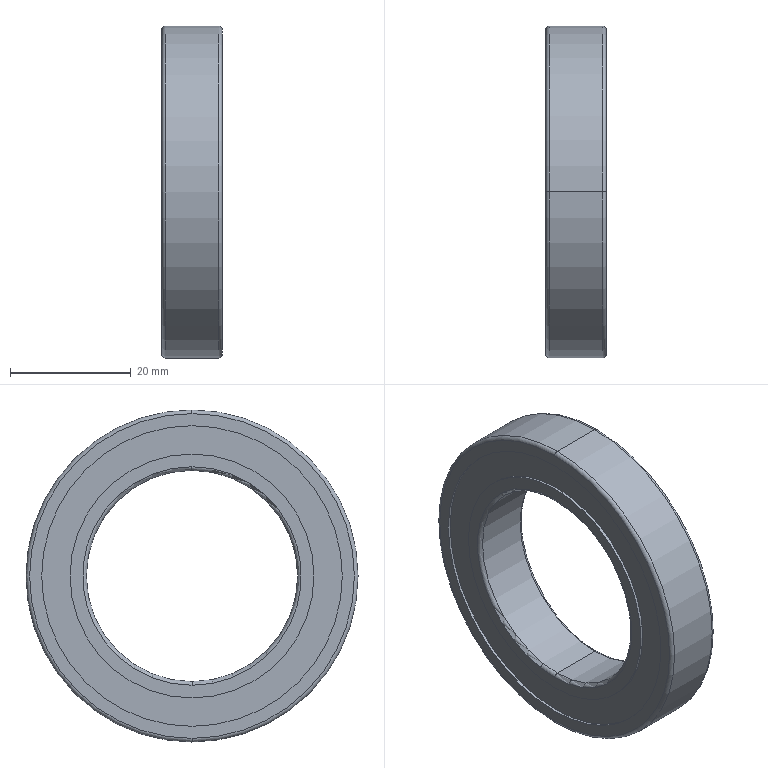Part | SolidWorks | features Fillet 2, Revolution 1 | 1 solid | 26 faces | box 10 x 55 x 55 mm | volume 13514 mm3 | cylinder 12 | torus 8 | plane 6 | commonest cylinder face diameters 40.4 x4 49.8 x4 35 x2 55 x2
STEP:
#1=CARTESIAN_POINT('',(0.6,0.,17.5));
#2=VERTEX_POINT('',#1);
#3=CARTESIAN_POINT('',(0.6,0.,-17.5));
#4=VERTEX_POINT('',#3);
#5=CARTESIAN_POINT('',(0.6,0.,0.));
#6=DIRECTION('',(-1.,0.,0.));
#7=DIRECTION('',(0.,0.,-1.));
#8=AXIS2_PLACEMENT_3D('',#5,#6,#7);
#9=CIRCLE('',#8,17.5);
#10=EDGE_CURVE('',#2,#4,#9,.T.);
#11=ORIENTED_EDGE('',*,*,#10,.F.);
#12=CARTESIAN_POINT('',(0.,0.,18.1));
#13=VERTEX_POINT('',#12);
#14=CARTESIAN_POINT('',(0.6,0.,18.1));
#15=DIRECTION('',(0.,1.,0.));
#16=DIRECTION('',(0.,0.,1.));
#17=AXIS2_PLACEMENT_3D('',#14,#15,#16);
#18=CIRCLE('',#17,0.6);
#19=EDGE_CURVE('',#2,#13,#18,.T.);
#20=ORIENTED_EDGE('',*,*,#19,.T.);
#21=CARTESIAN_POINT('',(0.,0.,-18.1));
#22=VERTEX_POINT('',#21);
#23=CARTESIAN_POINT('',(0.,0.,0.));
#24=DIRECTION('',(1.,0.,0.));
#25=DIRECTION('',(0.,0.,-1.));
#26=AXIS2_PLACEMENT_3D('',#23,#24,#25);
#27=CIRCLE('',#26,18.1);
#28=EDGE_CURVE('',#22,#13,#27,.T.);
#29=ORIENTED_EDGE('',*,*,#28,.F.);
#30=CARTESIAN_POINT('',(0.6,0.,-18.1));
#31=DIRECTION('',(0.,-1.,0.));
#32=DIRECTION('',(0.,0.,-1.));
#33=AXIS2_PLACEMENT_3D('',#30,#31,#32);
#34=CIRCLE('',#33,0.6);
#35=EDGE_CURVE('',#4,#22,#34,.T.);
#36=ORIENTED_EDGE('',*,*,#35,.F.);
#37=EDGE_LOOP('',(#11,#20,#29,#36));
#38=FACE_OUTER_BOUND('',#37,.T.);
#39=CARTESIAN_POINT('',(0.6,0.,0.));
#40=DIRECTION('',(1.,0.,0.));
#41=DIRECTION('',(0.,0.,-1.));
#42=AXIS2_PLACEMENT_3D('',#39,#40,#41);
#43=TOROIDAL_SURFACE('',#42,18.1,0.6);
#44=ADVANCED_FACE('',(#38),#43,.T.);
#45=CARTESIAN_POINT('',(9.4,0.,-17.5));
#46=VERTEX_POINT('',#45);
#47=CARTESIAN_POINT('',(9.4,0.,17.5));
#48=VERTEX_POINT('',#47);
#49=CARTESIAN_POINT('',(9.4,0.,0.));
#50=DIRECTION('',(1.,0.,0.));
#51=DIRECTION('',(0.,0.,1.));
#52=AXIS2_PLACEMENT_3D('',#49,#50,#51);
#53=CIRCLE('',#52,17.5);
#54=EDGE_CURVE('',#46,#48,#53,.T.);
#55=ORIENTED_EDGE('',*,*,#54,.F.);
#56=CARTESIAN_POINT('',(10.,0.,-18.1));
#57=VERTEX_POINT('',#56);
#58=CARTESIAN_POINT('',(9.4,0.,-18.1));
#59=DIRECTION('',(0.,1.,0.));
#60=DIRECTION('',(0.,0.,1.));
#61=AXIS2_PLACEMENT_3D('',#58,#59,#60);
#62=CIRCLE('',#61,0.6);
#63=EDGE_CURVE('',#46,#57,#62,.T.);
#64=ORIENTED_EDGE('',*,*,#63,.T.);
#65=CARTESIAN_POINT('',(10.,0.,18.1));
#66=VERTEX_POINT('',#65);
#67=CARTESIAN_POINT('',(10.,0.,0.));
#68=DIRECTION('',(-1.,0.,0.));
#69=DIRECTION('',(0.,0.,1.));
#70=AXIS2_PLACEMENT_3D('',#67,#68,#69);
#71=CIRCLE('',#70,18.1);
#72=EDGE_CURVE('',#66,#57,#71,.T.);
#73=ORIENTED_EDGE('',*,*,#72,.F.);
#74=CARTESIAN_POINT('',(9.4,0.,18.1));
#75=DIRECTION('',(0.,-1.,0.));
#76=DIRECTION('',(0.,0.,-1.));
#77=AXIS2_PLACEMENT_3D('',#74,#75,#76);
#78=CIRCLE('',#77,0.6);
#79=EDGE_CURVE('',#48,#66,#78,.T.);
#80=ORIENTED_EDGE('',*,*,#79,.F.);
#81=EDGE_LOOP('',(#55,#64,#73,#80));
#82=FACE_OUTER_BOUND('',#81,.T.);
#83=CARTESIAN_POINT('',(9.4,0.,0.));
#84=DIRECTION('',(-1.,0.,0.));
#85=DIRECTION('',(0.,0.,1.));
#86=AXIS2_PLACEMENT_3D('',#83,#84,#85);
#87=TOROIDAL_SURFACE('',#86,18.1,0.6);
#88=ADVANCED_FACE('',(#82),#87,.T.);
#89=CARTESIAN_POINT('',(0.,0.,26.9));
#90=VERTEX_POINT('',#89);
#91=CARTESIAN_POINT('',(0.,0.,-26.9));
#92=VERTEX_POINT('',#91);
#93=CARTESIAN_POINT('',(0.,0.,0.));
#94=DIRECTION('',(-1.,0.,0.));
#95=DIRECTION('',(0.,0.,-1.));
#96=AXIS2_PLACEMENT_3D('',#93,#94,#95);
#97=CIRCLE('',#96,26.9);
#98=EDGE_CURVE('',#90,#92,#97,.T.);
#99=ORIENTED_EDGE('',*,*,#98,.F.);
#100=CARTESIAN_POINT('',(0.6,0.,27.5));
#101=VERTEX_POINT('',#100);
#102=CARTESIAN_POINT('',(0.6,0.,26.9));
#103=DIRECTION('',(0.,1.,0.));
#104=DIRECTION('',(0.,0.,1.));
#105=AXIS2_PLACEMENT_3D('',#102,#103,#104);
#106=CIRCLE('',#105,0.6);
#107=EDGE_CURVE('',#90,#101,#106,.T.);
#108=ORIENTED_EDGE('',*,*,#107,.T.);
#109=CARTESIAN_POINT('',(0.6,0.,-27.5));
#110=VERTEX_POINT('',#109);
#111=CARTESIAN_POINT('',(0.6,0.,0.));
#112=DIRECTION('',(1.,0.,0.));
#113=DIRECTION('',(0.,0.,-1.));
#114=AXIS2_PLACEMENT_3D('',#111,#112,#113);
#115=CIRCLE('',#114,27.5);
#116=EDGE_CURVE('',#110,#101,#115,.T.);
#117=ORIENTED_EDGE('',*,*,#116,.F.);
#118=CARTESIAN_POINT('',(0.6,0.,-26.9));
#119=DIRECTION('',(0.,-1.,0.));
#120=DIRECTION('',(0.,0.,-1.));
#121=AXIS2_PLACEMENT_3D('',#118,#119,#120);
#122=CIRCLE('',#121,0.6);
#123=EDGE_CURVE('',#92,#110,#122,.T.);
#124=ORIENTED_EDGE('',*,*,#123,.F.);
#125=EDGE_LOOP('',(#99,#108,#117,#124));
#126=FACE_OUTER_BOUND('',#125,.T.);
#127=CARTESIAN_POINT('',(0.6,0.,0.));
#128=DIRECTION('',(1.,0.,0.));
#129=DIRECTION('',(0.,0.,-1.));
#130=AXIS2_PLACEMENT_3D('',#127,#128,#129);
#131=TOROIDAL_SURFACE('',#130,26.9,0.6);
#132=ADVANCED_FACE('',(#126),#131,.T.);
#133=CARTESIAN_POINT('',(10.,0.,-26.9));
#134=VERTEX_POINT('',#133);
#135=CARTESIAN_POINT('',(10.,0.,26.9));
#136=VERTEX_POINT('',#135);
#137=CARTESIAN_POINT('',(10.,0.,0.));
#138=DIRECTION('',(1.,0.,0.));
#139=DIRECTION('',(0.,0.,1.));
#140=AXIS2_PLACEMENT_3D('',#137,#138,#139);
#141=CIRCLE('',#140,26.9);
#142=EDGE_CURVE('',#134,#136,#141,.T.);
#143=ORIENTED_EDGE('',*,*,#142,.F.);
#144=CARTESIAN_POINT('',(9.4,0.,-27.5));
#145=VERTEX_POINT('',#144);
#146=CARTESIAN_POINT('',(9.4,0.,-26.9));
#147=DIRECTION('',(0.,1.,0.));
#148=DIRECTION('',(0.,0.,1.));
#149=AXIS2_PLACEMENT_3D('',#146,#147,#148);
#150=CIRCLE('',#149,0.6);
#151=EDGE_CURVE('',#134,#145,#150,.T.);
#152=ORIENTED_EDGE('',*,*,#151,.T.);
#153=CARTESIAN_POINT('',(9.4,0.,27.5));
#154=VERTEX_POINT('',#153);
#155=CARTESIAN_POINT('',(9.4,0.,0.));
#156=DIRECTION('',(-1.,0.,0.));
#157=DIRECTION('',(0.,0.,1.));
#158=AXIS2_PLACEMENT_3D('',#155,#156,#157);
#159=CIRCLE('',#158,27.5);
#160=EDGE_CURVE('',#154,#145,#159,.T.);
#161=ORIENTED_EDGE('',*,*,#160,.F.);
#162=CARTESIAN_POINT('',(9.4,0.,26.9));
#163=DIRECTION('',(0.,-1.,0.));
#164=DIRECTION('',(0.,0.,-1.));
#165=AXIS2_PLACEMENT_3D('',#162,#163,#164);
#166=CIRCLE('',#165,0.6);
#167=EDGE_CURVE('',#136,#154,#166,.T.);
#168=ORIENTED_EDGE('',*,*,#167,.F.);
#169=EDGE_LOOP('',(#143,#152,#161,#168));
#170=FACE_OUTER_BOUND('',#169,.T.);
#171=CARTESIAN_POINT('',(9.4,0.,0.));
#172=DIRECTION('',(-1.,0.,0.));
#173=DIRECTION('',(0.,0.,1.));
#174=AXIS2_PLACEMENT_3D('',#171,#172,#173);
#175=TOROIDAL_SURFACE('',#174,26.9,0.6);
#176=ADVANCED_FACE('',(#170),#175,.T.);
#177=ORIENTED_EDGE('',*,*,#160,.T.);
#178=CARTESIAN_POINT('',(0.,0.,-27.5));
#179=DIRECTION('',(-1.,0.,0.));
#180=VECTOR('',#179,1000.);
#181=LINE('',#178,#180);
#182=EDGE_CURVE('',#145,#110,#181,.T.);
#183=ORIENTED_EDGE('',*,*,#182,.T.);
#184=ORIENTED_EDGE('',*,*,#116,.T.);
#185=CARTESIAN_POINT('',(0.,0.,27.5));
#186=DIRECTION('',(-1.,0.,0.));
#187=VECTOR('',#186,1000.);
#188=LINE('',#185,#187);
#189=EDGE_CURVE('',#154,#101,#188,.T.);
#190=ORIENTED_EDGE('',*,*,#189,.F.);
#191=EDGE_LOOP('',(#177,#183,#184,#190));
#192=FACE_OUTER_BOUND('',#191,.T.);
#193=CARTESIAN_POINT('',(0.,0.,0.));
#194=DIRECTION('',(-1.,0.,0.));
#195=DIRECTION('',(0.,0.,1.));
#196=AXIS2_PLACEMENT_3D('',#193,#194,#195);
#197=CYLINDRICAL_SURFACE('',#196,27.5);
#198=ADVANCED_FACE('',(#192),#197,.T.);
#199=CARTESIAN_POINT('',(10.,0.,-24.9));
#200=VERTEX_POINT('',#199);
#201=CARTESIAN_POINT('',(10.,0.,24.9));
#202=VERTEX_POINT('',#201);
#203=CARTESIAN_POINT('',(10.,0.,0.));
#204=DIRECTION('',(-1.,0.,0.));
#205=DIRECTION('',(0.,0.,1.));
#206=AXIS2_PLACEMENT_3D('',#203,#204,#205);
#207=CIRCLE('',#206,24.9);
#208=EDGE_CURVE('',#200,#202,#207,.T.);
#209=ORIENTED_EDGE('',*,*,#208,.F.);
#210=CARTESIAN_POINT('',(9.565,0.,-24.9));
#211=VERTEX_POINT('',#210);
#212=CARTESIAN_POINT('',(0.,0.,-24.9));
#213=DIRECTION('',(-1.,0.,0.));
#214=VECTOR('',#213,1000.);
#215=LINE('',#212,#214);
#216=EDGE_CURVE('',#200,#211,#215,.T.);
#217=ORIENTED_EDGE('',*,*,#216,.T.);
#218=CARTESIAN_POINT('',(9.565,0.,24.9));
#219=VERTEX_POINT('',#218);
#220=CARTESIAN_POINT('',(9.565,0.,0.));
#221=DIRECTION('',(-1.,0.,0.));
#222=DIRECTION('',(0.,0.,1.));
#223=AXIS2_PLACEMENT_3D('',#220,#221,#222);
#224=CIRCLE('',#223,24.9);
#225=EDGE_CURVE('',#211,#219,#224,.T.);
#226=ORIENTED_EDGE('',*,*,#225,.T.);
#227=CARTESIAN_POINT('',(0.,0.,24.9));
#228=DIRECTION('',(-1.,0.,0.));
#229=VECTOR('',#228,1000.);
#230=LINE('',#227,#229);
#231=EDGE_CURVE('',#202,#219,#230,.T.);
#232=ORIENTED_EDGE('',*,*,#231,.F.);
#233=EDGE_LOOP('',(#209,#217,#226,#232));
#234=FACE_OUTER_BOUND('',#233,.T.);
#235=CARTESIAN_POINT('',(0.,0.,0.));
#236=DIRECTION('',(-1.,0.,0.));
#237=DIRECTION('',(0.,0.,1.));
#238=AXIS2_PLACEMENT_3D('',#235,#236,#237);
#239=CYLINDRICAL_SURFACE('',#238,24.9);
#240=ADVANCED_FACE('',(#234),#239,.F.);
#241=CARTESIAN_POINT('',(10.,0.,20.2));
#242=VERTEX_POINT('',#241);
#243=CARTESIAN_POINT('',(10.,0.,-20.2));
#244=VERTEX_POINT('',#243);
#245=CARTESIAN_POINT('',(10.,0.,0.));
#246=DIRECTION('',(-1.,0.,0.));
#247=DIRECTION('',(0.,0.,1.));
#248=AXIS2_PLACEMENT_3D('',#245,#246,#247);
#249=CIRCLE('',#248,20.2);
#250=EDGE_CURVE('',#242,#244,#249,.T.);
#251=ORIENTED_EDGE('',*,*,#250,.T.);
#252=CARTESIAN_POINT('',(9.565,0.,-20.2));
#253=VERTEX_POINT('',#252);
#254=CARTESIAN_POINT('',(0.,0.,-20.2));
#255=DIRECTION('',(-1.,0.,0.));
#256=VECTOR('',#255,1000.);
#257=LINE('',#254,#256);
#258=EDGE_CURVE('',#244,#253,#257,.T.);
#259=ORIENTED_EDGE('',*,*,#258,.T.);
#260=CARTESIAN_POINT('',(9.565,0.,20.2));
#261=VERTEX_POINT('',#260);
#262=CARTESIAN_POINT('',(9.565,0.,0.));
#263=DIRECTION('',(-1.,0.,0.));
#264=DIRECTION('',(0.,0.,1.));
#265=AXIS2_PLACEMENT_3D('',#262,#263,#264);
#266=CIRCLE('',#265,20.2);
#267=EDGE_CURVE('',#261,#253,#266,.T.);
#268=ORIENTED_EDGE('',*,*,#267,.F.);
#269=CARTESIAN_POINT('',(0.,0.,20.2));
#270=DIRECTION('',(-1.,0.,0.));
#271=VECTOR('',#270,1000.);
#272=LINE('',#269,#271);
#273=EDGE_CURVE('',#242,#261,#272,.T.);
#274=ORIENTED_EDGE('',*,*,#273,.F.);
#275=EDGE_LOOP('',(#251,#259,#268,#274));
#276=FACE_OUTER_BOUND('',#275,.T.);
#277=CARTESIAN_POINT('',(0.,0.,0.));
#278=DIRECTION('',(-1.,0.,0.));
#279=DIRECTION('',(0.,0.,1.));
#280=AXIS2_PLACEMENT_3D('',#277,#278,#279);
#281=CYLINDRICAL_SURFACE('',#280,20.2);
#282=ADVANCED_FACE('',(#276),#281,.T.);
#283=CARTESIAN_POINT('',(9.4,0.,0.));
#284=DIRECTION('',(1.,0.,0.));
#285=DIRECTION('',(0.,0.,1.));
#286=AXIS2_PLACEMENT_3D('',#283,#284,#285);
#287=CIRCLE('',#286,17.5);
#288=EDGE_CURVE('',#48,#46,#287,.T.);
#289=ORIENTED_EDGE('',*,*,#288,.T.);
#290=CARTESIAN_POINT('',(0.,0.,-17.5));
#291=DIRECTION('',(-1.,0.,0.));
#292=VECTOR('',#291,1000.);
#293=LINE('',#290,#292);
#294=EDGE_CURVE('',#46,#4,#293,.T.);
#295=ORIENTED_EDGE('',*,*,#294,.T.);
#296=CARTESIAN_POINT('',(0.6,0.,0.));
#297=DIRECTION('',(-1.,0.,0.));
#298=DIRECTION('',(0.,0.,-1.));
#299=AXIS2_PLACEMENT_3D('',#296,#297,#298);
#300=CIRCLE('',#299,17.5);
#301=EDGE_CURVE('',#4,#2,#300,.T.);
#302=ORIENTED_EDGE('',*,*,#301,.T.);
#303=CARTESIAN_POINT('',(0.,0.,17.5));
#304=DIRECTION('',(-1.,0.,0.));
#305=VECTOR('',#304,1000.);
#306=LINE('',#303,#305);
#307=EDGE_CURVE('',#48,#2,#306,.T.);
#308=ORIENTED_EDGE('',*,*,#307,.F.);
#309=EDGE_LOOP('',(#289,#295,#302,#308));
#310=FACE_OUTER_BOUND('',#309,.T.);
#311=CARTESIAN_POINT('',(0.,0.,0.));
#312=DIRECTION('',(-1.,0.,0.));
#313=DIRECTION('',(0.,0.,1.));
#314=AXIS2_PLACEMENT_3D('',#311,#312,#313);
#315=CYLINDRICAL_SURFACE('',#314,17.5);
#316=ADVANCED_FACE('',(#310),#315,.F.);
#317=CARTESIAN_POINT('',(0.435,0.,20.2));
#318=VERTEX_POINT('',#317);
#319=CARTESIAN_POINT('',(0.435,0.,-20.2));
#320=VERTEX_POINT('',#319);
#321=CARTESIAN_POINT('',(0.435,0.,0.));
#322=DIRECTION('',(-1.,0.,0.));
#323=DIRECTION('',(0.,0.,1.));
#324=AXIS2_PLACEMENT_3D('',#321,#322,#323);
#325=CIRCLE('',#324,20.2);
#326=EDGE_CURVE('',#318,#320,#325,.T.);
#327=ORIENTED_EDGE('',*,*,#326,.T.);
#328=CARTESIAN_POINT('',(0.,0.,-20.2));
#329=VERTEX_POINT('',#328);
#330=CARTESIAN_POINT('',(0.,0.,-20.2));
#331=DIRECTION('',(-1.,0.,0.));
#332=VECTOR('',#331,1000.);
#333=LINE('',#330,#332);
#334=EDGE_CURVE('',#320,#329,#333,.T.);
#335=ORIENTED_EDGE('',*,*,#334,.T.);
#336=CARTESIAN_POINT('',(0.,0.,20.2));
#337=VERTEX_POINT('',#336);
#338=CARTESIAN_POINT('',(0.,0.,0.));
#339=DIRECTION('',(-1.,0.,0.));
#340=DIRECTION('',(0.,0.,1.));
#341=AXIS2_PLACEMENT_3D('',#338,#339,#340);
#342=CIRCLE('',#341,20.2);
#343=EDGE_CURVE('',#337,#329,#342,.T.);
#344=ORIENTED_EDGE('',*,*,#343,.F.);
#345=CARTESIAN_POINT('',(0.,0.,20.2));
#346=DIRECTION('',(-1.,0.,0.));
#347=VECTOR('',#346,1000.);
#348=LINE('',#345,#347);
#349=EDGE_CURVE('',#318,#337,#348,.T.);
#350=ORIENTED_EDGE('',*,*,#349,.F.);
#351=EDGE_LOOP('',(#327,#335,#344,#350));
#352=FACE_OUTER_BOUND('',#351,.T.);
#353=CARTESIAN_POINT('',(0.,0.,0.));
#354=DIRECTION('',(-1.,0.,0.));
#355=DIRECTION('',(0.,0.,1.));
#356=AXIS2_PLACEMENT_3D('',#353,#354,#355);
#357=CYLINDRICAL_SURFACE('',#356,20.2);
#358=ADVANCED_FACE('',(#352),#357,.T.);
#359=CARTESIAN_POINT('',(0.435,0.,-24.9));
#360=VERTEX_POINT('',#359);
#361=CARTESIAN_POINT('',(0.435,0.,24.9));
#362=VERTEX_POINT('',#361);
#363=CARTESIAN_POINT('',(0.435,0.,0.));
#364=DIRECTION('',(-1.,0.,0.));
#365=DIRECTION('',(0.,0.,1.));
#366=AXIS2_PLACEMENT_3D('',#363,#364,#365);
#367=CIRCLE('',#366,24.9);
#368=EDGE_CURVE('',#360,#362,#367,.T.);
#369=ORIENTED_EDGE('',*,*,#368,.F.);
#370=CARTESIAN_POINT('',(0.,0.,-24.9));
#371=VERTEX_POINT('',#370);
#372=CARTESIAN_POINT('',(0.,0.,-24.9));
#373=DIRECTION('',(-1.,0.,0.));
#374=VECTOR('',#373,1000.);
#375=LINE('',#372,#374);
#376=EDGE_CURVE('',#360,#371,#375,.T.);
#377=ORIENTED_EDGE('',*,*,#376,.T.);
#378=CARTESIAN_POINT('',(0.,0.,24.9));
#379=VERTEX_POINT('',#378);
#380=CARTESIAN_POINT('',(0.,0.,0.));
#381=DIRECTION('',(-1.,0.,0.));
#382=DIRECTION('',(0.,0.,1.));
#383=AXIS2_PLACEMENT_3D('',#380,#381,#382);
#384=CIRCLE('',#383,24.9);
#385=EDGE_CURVE('',#371,#379,#384,.T.);
#386=ORIENTED_EDGE('',*,*,#385,.T.);
#387=CARTESIAN_POINT('',(0.,0.,24.9));
#388=DIRECTION('',(-1.,0.,0.));
#389=VECTOR('',#388,1000.);
#390=LINE('',#387,#389);
#391=EDGE_CURVE('',#362,#379,#390,.T.);
#392=ORIENTED_EDGE('',*,*,#391,.F.);
#393=EDGE_LOOP('',(#369,#377,#386,#392));
#394=FACE_OUTER_BOUND('',#393,.T.);
#395=CARTESIAN_POINT('',(0.,0.,0.));
#396=DIRECTION('',(-1.,0.,0.));
#397=DIRECTION('',(0.,0.,1.));
#398=AXIS2_PLACEMENT_3D('',#395,#396,#397);
#399=CYLINDRICAL_SURFACE('',#398,24.9);
#400=ADVANCED_FACE('',(#394),#399,.F.);
#401=CARTESIAN_POINT('',(0.,0.,0.));
#402=DIRECTION('',(-1.,0.,0.));
#403=DIRECTION('',(0.,0.,-1.));
#404=AXIS2_PLACEMENT_3D('',#401,#402,#403);
#405=CIRCLE('',#404,26.9);
#406=EDGE_CURVE('',#92,#90,#405,.T.);
#407=ORIENTED_EDGE('',*,*,#406,.T.);
#408=ORIENTED_EDGE('',*,*,#98,.T.);
#409=EDGE_LOOP('',(#407,#408));
#410=FACE_OUTER_BOUND('',#409,.T.);
#411=CARTESIAN_POINT('',(0.,0.,0.));
#412=DIRECTION('',(-1.,0.,0.));
#413=DIRECTION('',(0.,0.,1.));
#414=AXIS2_PLACEMENT_3D('',#411,#412,#413);
#415=CIRCLE('',#414,24.9);
#416=EDGE_CURVE('',#379,#371,#415,.T.);
#417=ORIENTED_EDGE('',*,*,#416,.F.);
#418=ORIENTED_EDGE('',*,*,#385,.F.);
#419=EDGE_LOOP('',(#417,#418));
#420=FACE_BOUND('',#419,.T.);
#421=CARTESIAN_POINT('',(0.,27.5,0.));
#422=DIRECTION('',(1.,0.,0.));
#423=DIRECTION('',(0.,0.,-1.));
#424=AXIS2_PLACEMENT_3D('',#421,#422,#423);
#425=PLANE('',#424);
#426=ADVANCED_FACE('',(#410,#420),#425,.F.);
#427=ORIENTED_EDGE('',*,*,#376,.F.);
#428=CARTESIAN_POINT('',(0.435,0.,0.));
#429=DIRECTION('',(-1.,0.,0.));
#430=DIRECTION('',(0.,0.,1.));
#431=AXIS2_PLACEMENT_3D('',#428,#429,#430);
#432=CIRCLE('',#431,24.9);
#433=EDGE_CURVE('',#362,#360,#432,.T.);
#434=ORIENTED_EDGE('',*,*,#433,.F.);
#435=ORIENTED_EDGE('',*,*,#391,.T.);
#436=ORIENTED_EDGE('',*,*,#416,.T.);
#437=EDGE_LOOP('',(#427,#434,#435,#436));
#438=FACE_OUTER_BOUND('',#437,.T.);
#439=CARTESIAN_POINT('',(0.,0.,0.));
#440=DIRECTION('',(-1.,0.,0.));
#441=DIRECTION('',(0.,0.,1.));
#442=AXIS2_PLACEMENT_3D('',#439,#440,#441);
#443=CYLINDRICAL_SURFACE('',#442,24.9);
#444=ADVANCED_FACE('',(#438),#443,.F.);
#445=ORIENTED_EDGE('',*,*,#326,.F.);
#446=CARTESIAN_POINT('',(0.435,0.,0.));
#447=DIRECTION('',(-1.,0.,0.));
#448=DIRECTION('',(0.,0.,1.));
#449=AXIS2_PLACEMENT_3D('',#446,#447,#448);
#450=CIRCLE('',#449,20.2);
#451=EDGE_CURVE('',#320,#318,#450,.T.);
#452=ORIENTED_EDGE('',*,*,#451,.F.);
#453=EDGE_LOOP('',(#445,#452));
#454=FACE_BOUND('',#453,.T.);
#455=ORIENTED_EDGE('',*,*,#433,.T.);
#456=ORIENTED_EDGE('',*,*,#368,.T.);
#457=EDGE_LOOP('',(#455,#456));
#458=FACE_OUTER_BOUND('',#457,.T.);
#459=CARTESIAN_POINT('',(0.435,24.9,0.));
#460=DIRECTION('',(1.,0.,0.));
#461=DIRECTION('',(0.,0.,-1.));
#462=AXIS2_PLACEMENT_3D('',#459,#460,#461);
#463=PLANE('',#462);
#464=ADVANCED_FACE('',(#454,#458),#463,.F.);
#465=ORIENTED_EDGE('',*,*,#334,.F.);
#466=ORIENTED_EDGE('',*,*,#451,.T.);
#467=ORIENTED_EDGE('',*,*,#349,.T.);
#468=CARTESIAN_POINT('',(0.,0.,0.));
#469=DIRECTION('',(-1.,0.,0.));
#470=DIRECTION('',(0.,0.,1.));
#471=AXIS2_PLACEMENT_3D('',#468,#469,#470);
#472=CIRCLE('',#471,20.2);
#473=EDGE_CURVE('',#329,#337,#472,.T.);
#474=ORIENTED_EDGE('',*,*,#473,.F.);
#475=EDGE_LOOP('',(#465,#466,#467,#474));
#476=FACE_OUTER_BOUND('',#475,.T.);
#477=CARTESIAN_POINT('',(0.,0.,0.));
#478=DIRECTION('',(-1.,0.,0.));
#479=DIRECTION('',(0.,0.,1.));
#480=AXIS2_PLACEMENT_3D('',#477,#478,#479);
#481=CYLINDRICAL_SURFACE('',#480,20.2);
#482=ADVANCED_FACE('',(#476),#481,.T.);
#483=ORIENTED_EDGE('',*,*,#28,.T.);
#484=CARTESIAN_POINT('',(0.,0.,0.));
#485=DIRECTION('',(1.,0.,0.));
#486=DIRECTION('',(0.,0.,-1.));
#487=AXIS2_PLACEMENT_3D('',#484,#485,#486);
#488=CIRCLE('',#487,18.1);
#489=EDGE_CURVE('',#13,#22,#488,.T.);
#490=ORIENTED_EDGE('',*,*,#489,.T.);
#491=EDGE_LOOP('',(#483,#490));
#492=FACE_BOUND('',#491,.T.);
#493=ORIENTED_EDGE('',*,*,#343,.T.);
#494=ORIENTED_EDGE('',*,*,#473,.T.);
#495=EDGE_LOOP('',(#493,#494));
#496=FACE_OUTER_BOUND('',#495,.T.);
#497=CARTESIAN_POINT('',(0.,20.2,0.));
#498=DIRECTION('',(1.,0.,0.));
#499=DIRECTION('',(0.,0.,-1.));
#500=AXIS2_PLACEMENT_3D('',#497,#498,#499);
#501=PLANE('',#500);
#502=ADVANCED_FACE('',(#492,#496),#501,.F.);
#503=ORIENTED_EDGE('',*,*,#294,.F.);
#504=ORIENTED_EDGE('',*,*,#54,.T.);
#505=ORIENTED_EDGE('',*,*,#307,.T.);
#506=ORIENTED_EDGE('',*,*,#10,.T.);
#507=EDGE_LOOP('',(#503,#504,#505,#506));
#508=FACE_OUTER_BOUND('',#507,.T.);
#509=CARTESIAN_POINT('',(0.,0.,0.));
#510=DIRECTION('',(-1.,0.,0.));
#511=DIRECTION('',(0.,0.,1.));
#512=AXIS2_PLACEMENT_3D('',#509,#510,#511);
#513=CYLINDRICAL_SURFACE('',#512,17.5);
#514=ADVANCED_FACE('',(#508),#513,.F.);
#515=ORIENTED_EDGE('',*,*,#72,.T.);
#516=CARTESIAN_POINT('',(10.,0.,0.));
#517=DIRECTION('',(-1.,0.,0.));
#518=DIRECTION('',(0.,0.,1.));
#519=AXIS2_PLACEMENT_3D('',#516,#517,#518);
#520=CIRCLE('',#519,18.1);
#521=EDGE_CURVE('',#57,#66,#520,.T.);
#522=ORIENTED_EDGE('',*,*,#521,.T.);
#523=EDGE_LOOP('',(#515,#522));
#524=FACE_BOUND('',#523,.T.);
#525=ORIENTED_EDGE('',*,*,#250,.F.);
#526=CARTESIAN_POINT('',(10.,0.,0.));
#527=DIRECTION('',(-1.,0.,0.));
#528=DIRECTION('',(0.,0.,1.));
#529=AXIS2_PLACEMENT_3D('',#526,#527,#528);
#530=CIRCLE('',#529,20.2);
#531=EDGE_CURVE('',#244,#242,#530,.T.);
#532=ORIENTED_EDGE('',*,*,#531,.F.);
#533=EDGE_LOOP('',(#525,#532));
#534=FACE_OUTER_BOUND('',#533,.T.);
#535=CARTESIAN_POINT('',(10.,20.2,0.));
#536=DIRECTION('',(-1.,0.,0.));
#537=DIRECTION('',(0.,0.,1.));
#538=AXIS2_PLACEMENT_3D('',#535,#536,#537);
#539=PLANE('',#538);
#540=ADVANCED_FACE('',(#524,#534),#539,.F.);
#541=ORIENTED_EDGE('',*,*,#258,.F.);
#542=ORIENTED_EDGE('',*,*,#531,.T.);
#543=ORIENTED_EDGE('',*,*,#273,.T.);
#544=CARTESIAN_POINT('',(9.565,0.,0.));
#545=DIRECTION('',(-1.,0.,0.));
#546=DIRECTION('',(0.,0.,1.));
#547=AXIS2_PLACEMENT_3D('',#544,#545,#546);
#548=CIRCLE('',#547,20.2);
#549=EDGE_CURVE('',#253,#261,#548,.T.);
#550=ORIENTED_EDGE('',*,*,#549,.F.);
#551=EDGE_LOOP('',(#541,#542,#543,#550));
#552=FACE_OUTER_BOUND('',#551,.T.);
#553=CARTESIAN_POINT('',(0.,0.,0.));
#554=DIRECTION('',(-1.,0.,0.));
#555=DIRECTION('',(0.,0.,1.));
#556=AXIS2_PLACEMENT_3D('',#553,#554,#555);
#557=CYLINDRICAL_SURFACE('',#556,20.2);
#558=ADVANCED_FACE('',(#552),#557,.T.);
#559=CARTESIAN_POINT('',(9.565,0.,0.));
#560=DIRECTION('',(-1.,0.,0.));
#561=DIRECTION('',(0.,0.,1.));
#562=AXIS2_PLACEMENT_3D('',#559,#560,#561);
#563=CIRCLE('',#562,24.9);
#564=EDGE_CURVE('',#219,#211,#563,.T.);
#565=ORIENTED_EDGE('',*,*,#564,.F.);
#566=ORIENTED_EDGE('',*,*,#225,.F.);
#567=EDGE_LOOP('',(#565,#566));
#568=FACE_OUTER_BOUND('',#567,.T.);
#569=ORIENTED_EDGE('',*,*,#267,.T.);
#570=ORIENTED_EDGE('',*,*,#549,.T.);
#571=EDGE_LOOP('',(#569,#570));
#572=FACE_BOUND('',#571,.T.);
#573=CARTESIAN_POINT('',(9.565,24.9,0.));
#574=DIRECTION('',(-1.,0.,0.));
#575=DIRECTION('',(0.,0.,1.));
#576=AXIS2_PLACEMENT_3D('',#573,#574,#575);
#577=PLANE('',#576);
#578=ADVANCED_FACE('',(#568,#572),#577,.F.);
#579=ORIENTED_EDGE('',*,*,#216,.F.);
#580=CARTESIAN_POINT('',(10.,0.,0.));
#581=DIRECTION('',(-1.,0.,0.));
#582=DIRECTION('',(0.,0.,1.));
#583=AXIS2_PLACEMENT_3D('',#580,#581,#582);
#584=CIRCLE('',#583,24.9);
#585=EDGE_CURVE('',#202,#200,#584,.T.);
#586=ORIENTED_EDGE('',*,*,#585,.F.);
#587=ORIENTED_EDGE('',*,*,#231,.T.);
#588=ORIENTED_EDGE('',*,*,#564,.T.);
#589=EDGE_LOOP('',(#579,#586,#587,#588));
#590=FACE_OUTER_BOUND('',#589,.T.);
#591=CARTESIAN_POINT('',(0.,0.,0.));
#592=DIRECTION('',(-1.,0.,0.));
#593=DIRECTION('',(0.,0.,1.));
#594=AXIS2_PLACEMENT_3D('',#591,#592,#593);
#595=CYLINDRICAL_SURFACE('',#594,24.9);
#596=ADVANCED_FACE('',(#590),#595,.F.);
#597=CARTESIAN_POINT('',(10.,0.,0.));
#598=DIRECTION('',(1.,0.,0.));
#599=DIRECTION('',(0.,0.,1.));
#600=AXIS2_PLACEMENT_3D('',#597,#598,#599);
#601=CIRCLE('',#600,26.9);
#602=EDGE_CURVE('',#136,#134,#601,.T.);
#603=ORIENTED_EDGE('',*,*,#602,.T.);
#604=ORIENTED_EDGE('',*,*,#142,.T.);
#605=EDGE_LOOP('',(#603,#604));
#606=FACE_OUTER_BOUND('',#605,.T.);
#607=ORIENTED_EDGE('',*,*,#585,.T.);
#608=ORIENTED_EDGE('',*,*,#208,.T.);
#609=EDGE_LOOP('',(#607,#608));
#610=FACE_BOUND('',#609,.T.);
#611=CARTESIAN_POINT('',(10.,27.5,0.));
#612=DIRECTION('',(-1.,0.,0.));
#613=DIRECTION('',(0.,0.,1.));
#614=AXIS2_PLACEMENT_3D('',#611,#612,#613);
#615=PLANE('',#614);
#616=ADVANCED_FACE('',(#606,#610),#615,.F.);
#617=ORIENTED_EDGE('',*,*,#182,.F.);
#618=CARTESIAN_POINT('',(9.4,0.,0.));
#619=DIRECTION('',(-1.,0.,0.));
#620=DIRECTION('',(0.,0.,1.));
#621=AXIS2_PLACEMENT_3D('',#618,#619,#620);
#622=CIRCLE('',#621,27.5);
#623=EDGE_CURVE('',#145,#154,#622,.T.);
#624=ORIENTED_EDGE('',*,*,#623,.T.);
#625=ORIENTED_EDGE('',*,*,#189,.T.);
#626=CARTESIAN_POINT('',(0.6,0.,0.));
#627=DIRECTION('',(1.,0.,0.));
#628=DIRECTION('',(0.,0.,-1.));
#629=AXIS2_PLACEMENT_3D('',#626,#627,#628);
#630=CIRCLE('',#629,27.5);
#631=EDGE_CURVE('',#101,#110,#630,.T.);
#632=ORIENTED_EDGE('',*,*,#631,.T.);
#633=EDGE_LOOP('',(#617,#624,#625,#632));
#634=FACE_OUTER_BOUND('',#633,.T.);
#635=CARTESIAN_POINT('',(0.,0.,0.));
#636=DIRECTION('',(-1.,0.,0.));
#637=DIRECTION('',(0.,0.,1.));
#638=AXIS2_PLACEMENT_3D('',#635,#636,#637);
#639=CYLINDRICAL_SURFACE('',#638,27.5);
#640=ADVANCED_FACE('',(#634),#639,.T.);
#641=ORIENTED_EDGE('',*,*,#151,.F.);
#642=ORIENTED_EDGE('',*,*,#602,.F.);
#643=ORIENTED_EDGE('',*,*,#167,.T.);
#644=ORIENTED_EDGE('',*,*,#623,.F.);
#645=EDGE_LOOP('',(#641,#642,#643,#644));
#646=FACE_OUTER_BOUND('',#645,.T.);
#647=CARTESIAN_POINT('',(9.4,0.,0.));
#648=DIRECTION('',(-1.,0.,0.));
#649=DIRECTION('',(0.,0.,1.));
#650=AXIS2_PLACEMENT_3D('',#647,#648,#649);
#651=TOROIDAL_SURFACE('',#650,26.9,0.6);
#652=ADVANCED_FACE('',(#646),#651,.T.);
#653=ORIENTED_EDGE('',*,*,#107,.F.);
#654=ORIENTED_EDGE('',*,*,#406,.F.);
#655=ORIENTED_EDGE('',*,*,#123,.T.);
#656=ORIENTED_EDGE('',*,*,#631,.F.);
#657=EDGE_LOOP('',(#653,#654,#655,#656));
#658=FACE_OUTER_BOUND('',#657,.T.);
#659=CARTESIAN_POINT('',(0.6,0.,0.));
#660=DIRECTION('',(1.,0.,0.));
#661=DIRECTION('',(0.,0.,-1.));
#662=AXIS2_PLACEMENT_3D('',#659,#660,#661);
#663=TOROIDAL_SURFACE('',#662,26.9,0.6);
#664=ADVANCED_FACE('',(#658),#663,.T.);
#665=ORIENTED_EDGE('',*,*,#63,.F.);
#666=ORIENTED_EDGE('',*,*,#288,.F.);
#667=ORIENTED_EDGE('',*,*,#79,.T.);
#668=ORIENTED_EDGE('',*,*,#521,.F.);
#669=EDGE_LOOP('',(#665,#666,#667,#668));
#670=FACE_OUTER_BOUND('',#669,.T.);
#671=CARTESIAN_POINT('',(9.4,0.,0.));
#672=DIRECTION('',(-1.,0.,0.));
#673=DIRECTION('',(0.,0.,1.));
#674=AXIS2_PLACEMENT_3D('',#671,#672,#673);
#675=TOROIDAL_SURFACE('',#674,18.1,0.6);
#676=ADVANCED_FACE('',(#670),#675,.T.);
#677=ORIENTED_EDGE('',*,*,#19,.F.);
#678=ORIENTED_EDGE('',*,*,#301,.F.);
#679=ORIENTED_EDGE('',*,*,#35,.T.);
#680=ORIENTED_EDGE('',*,*,#489,.F.);
#681=EDGE_LOOP('',(#677,#678,#679,#680));
#682=FACE_OUTER_BOUND('',#681,.T.);
#683=CARTESIAN_POINT('',(0.6,0.,0.));
#684=DIRECTION('',(1.,0.,0.));
#685=DIRECTION('',(0.,0.,-1.));
#686=AXIS2_PLACEMENT_3D('',#683,#684,#685);
#687=TOROIDAL_SURFACE('',#686,18.1,0.6);
#688=ADVANCED_FACE('',(#682),#687,.T.);
#689=CLOSED_SHELL('',(#44,#88,#132,#176,#198,#240,#282,#316,#358,#400,#426,#444,#464,#482,#502,#514,#540,#558,#578,#596,#616,#640,#652,#664,#676,#688));
#690=MANIFOLD_SOLID_BREP('',#689);
#691=CARTESIAN_POINT('',(0.,0.,0.));
#692=DIRECTION('',(0.,0.,1.));
#693=DIRECTION('',(1.,0.,0.));
#694=AXIS2_PLACEMENT_3D('',#691,#692,#693);
#695=(LENGTH_UNIT()NAMED_UNIT(*)SI_UNIT(.MILLI.,.METRE.));
#696=UNCERTAINTY_MEASURE_WITH_UNIT(LENGTH_MEASURE(0.00001),#695,'','');
#697=(NAMED_UNIT(*)PLANE_ANGLE_UNIT()SI_UNIT($,.RADIAN.));
#698=(NAMED_UNIT(*)SI_UNIT($,.STERADIAN.)SOLID_ANGLE_UNIT());
#699=(GEOMETRIC_REPRESENTATION_CONTEXT(3)GLOBAL_UNCERTAINTY_ASSIGNED_CONTEXT((#696))GLOBAL_UNIT_ASSIGNED_CONTEXT((#695,#697,#698))REPRESENTATION_CONTEXT('',''));
#700=ADVANCED_BREP_SHAPE_REPRESENTATION('',(#690,#694),#699);